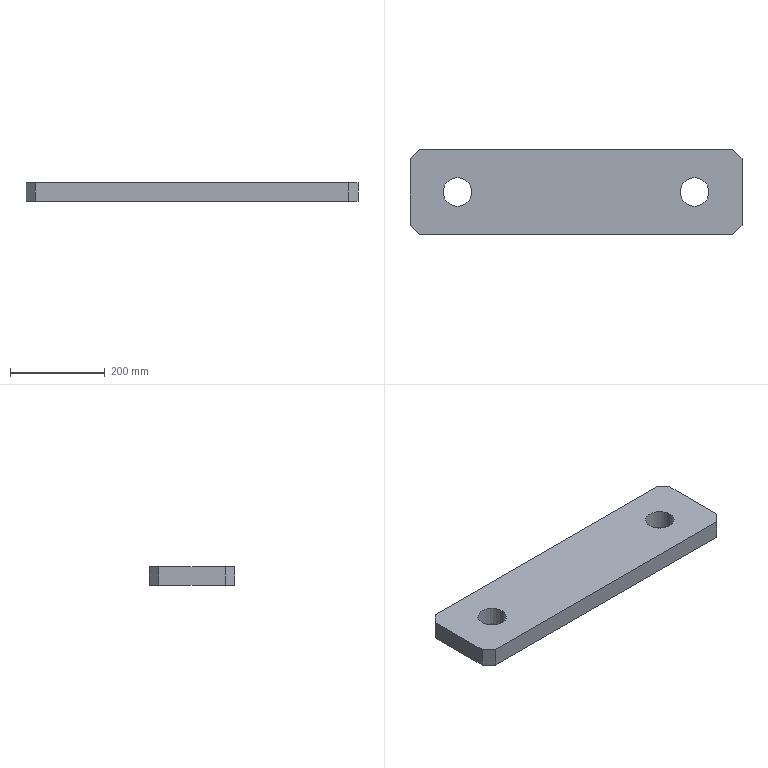Part | STEP file | 001-009-Riveting base plate | 1 solid | 14 faces | box 700 x 180 x 40 mm | volume 4781805 mm3 | plane 10 | cylinder 4 | commonest cylinder face diameters 60 x4
STEP:
#1=CARTESIAN_POINT('',(0.,0.,0.));
#2=DIRECTION('',(0.,0.,1.));
#3=DIRECTION('',(1.,0.,0.));
#4=AXIS2_PLACEMENT_3D('',#1,#2,#3);
#5=CARTESIAN_POINT('',(220.,0.,40.));
#6=VERTEX_POINT('',#5);
#7=CARTESIAN_POINT('',(220.,0.,0.));
#8=VERTEX_POINT('',#7);
#9=CARTESIAN_POINT('',(220.,0.,40.));
#10=DIRECTION('',(0.,0.,-1.));
#11=VECTOR('',#10,1.);
#12=LINE('',#9,#11);
#13=CARTESIAN_POINT('',(250.,0.,40.));
#14=DIRECTION('',(0.,0.,-1.));
#15=DIRECTION('',(-1.,0.,0.));
#16=AXIS2_PLACEMENT_3D('',#13,#14,#15);
#17=CYLINDRICAL_SURFACE('',#16,30.);
#18=CARTESIAN_POINT('',(6.283,0.));
#19=DIRECTION('',(0.,1.));
#20=VECTOR('',#19,1.);
#21=LINE('',#18,#20);
#22=(GEOMETRIC_REPRESENTATION_CONTEXT(2)PARAMETRIC_REPRESENTATION_CONTEXT()REPRESENTATION_CONTEXT('',''));
#23=DEFINITIONAL_REPRESENTATION('',(#21),#22);
#24=PCURVE('',#17,#23);
#25=CARTESIAN_POINT('',(250.,0.,40.));
#26=DIRECTION('',(0.,0.,-1.));
#27=DIRECTION('',(-1.,0.,0.));
#28=AXIS2_PLACEMENT_3D('',#25,#26,#27);
#29=CYLINDRICAL_SURFACE('',#28,30.);
#30=CARTESIAN_POINT('',(0.,0.));
#31=DIRECTION('',(0.,1.));
#32=VECTOR('',#31,1.);
#33=LINE('',#30,#32);
#34=(GEOMETRIC_REPRESENTATION_CONTEXT(2)PARAMETRIC_REPRESENTATION_CONTEXT()REPRESENTATION_CONTEXT('',''));
#35=DEFINITIONAL_REPRESENTATION('',(#33),#34);
#36=PCURVE('',#29,#35);
#37=SURFACE_CURVE('',#12,(#24,#36),.PCURVE_S1.);
#38=EDGE_CURVE('',#6,#8,#37,.T.);
#39=ORIENTED_EDGE('',*,*,#38,.T.);
#40=CARTESIAN_POINT('',(280.,0.,0.));
#41=VERTEX_POINT('',#40);
#42=CARTESIAN_POINT('',(250.,0.,0.));
#43=DIRECTION('',(0.,0.,-1.));
#44=DIRECTION('',(-1.,0.,0.));
#45=AXIS2_PLACEMENT_3D('',#42,#43,#44);
#46=CIRCLE('',#45,30.);
#47=CARTESIAN_POINT('',(0.,40.));
#48=DIRECTION('',(1.,0.));
#49=VECTOR('',#48,1.);
#50=LINE('',#47,#49);
#51=(GEOMETRIC_REPRESENTATION_CONTEXT(2)PARAMETRIC_REPRESENTATION_CONTEXT()REPRESENTATION_CONTEXT('',''));
#52=DEFINITIONAL_REPRESENTATION('',(#50),#51);
#53=PCURVE('',#17,#52);
#54=CARTESIAN_POINT('',(0.,0.,0.));
#55=DIRECTION('',(0.,0.,-1.));
#56=DIRECTION('',(-1.,0.,0.));
#57=AXIS2_PLACEMENT_3D('',#54,#55,#56);
#58=PLANE('',#57);
#59=CARTESIAN_POINT('',(-250.,0.));
#60=DIRECTION('',(1.,0.));
#61=AXIS2_PLACEMENT_2D('',#59,#60);
#62=CIRCLE('',#61,30.);
#63=(GEOMETRIC_REPRESENTATION_CONTEXT(2)PARAMETRIC_REPRESENTATION_CONTEXT()REPRESENTATION_CONTEXT('',''));
#64=DEFINITIONAL_REPRESENTATION('',(#62),#63);
#65=PCURVE('',#58,#64);
#66=SURFACE_CURVE('',#46,(#53,#65),.PCURVE_S1.);
#67=EDGE_CURVE('',#41,#8,#66,.T.);
#68=ORIENTED_EDGE('',*,*,#67,.F.);
#69=CARTESIAN_POINT('',(280.,0.,40.));
#70=VERTEX_POINT('',#69);
#71=CARTESIAN_POINT('',(280.,0.,40.));
#72=DIRECTION('',(0.,0.,-1.));
#73=VECTOR('',#72,1.);
#74=LINE('',#71,#73);
#75=CARTESIAN_POINT('',(3.142,0.));
#76=DIRECTION('',(0.,1.));
#77=VECTOR('',#76,1.);
#78=LINE('',#75,#77);
#79=(GEOMETRIC_REPRESENTATION_CONTEXT(2)PARAMETRIC_REPRESENTATION_CONTEXT()REPRESENTATION_CONTEXT('',''));
#80=DEFINITIONAL_REPRESENTATION('',(#78),#79);
#81=PCURVE('',#17,#80);
#82=CARTESIAN_POINT('',(3.142,0.));
#83=DIRECTION('',(0.,1.));
#84=VECTOR('',#83,1.);
#85=LINE('',#82,#84);
#86=(GEOMETRIC_REPRESENTATION_CONTEXT(2)PARAMETRIC_REPRESENTATION_CONTEXT()REPRESENTATION_CONTEXT('',''));
#87=DEFINITIONAL_REPRESENTATION('',(#85),#86);
#88=PCURVE('',#29,#87);
#89=SURFACE_CURVE('',#74,(#81,#88),.PCURVE_S1.);
#90=EDGE_CURVE('',#70,#41,#89,.T.);
#91=ORIENTED_EDGE('',*,*,#90,.F.);
#92=CARTESIAN_POINT('',(250.,0.,40.));
#93=DIRECTION('',(0.,0.,-1.));
#94=DIRECTION('',(-1.,0.,0.));
#95=AXIS2_PLACEMENT_3D('',#92,#93,#94);
#96=CIRCLE('',#95,30.);
#97=CARTESIAN_POINT('',(0.,0.));
#98=DIRECTION('',(1.,0.));
#99=VECTOR('',#98,1.);
#100=LINE('',#97,#99);
#101=(GEOMETRIC_REPRESENTATION_CONTEXT(2)PARAMETRIC_REPRESENTATION_CONTEXT()REPRESENTATION_CONTEXT('',''));
#102=DEFINITIONAL_REPRESENTATION('',(#100),#101);
#103=PCURVE('',#17,#102);
#104=CARTESIAN_POINT('',(0.,0.,40.));
#105=DIRECTION('',(0.,0.,-1.));
#106=DIRECTION('',(-1.,0.,0.));
#107=AXIS2_PLACEMENT_3D('',#104,#105,#106);
#108=PLANE('',#107);
#109=CARTESIAN_POINT('',(-250.,0.));
#110=DIRECTION('',(1.,0.));
#111=AXIS2_PLACEMENT_2D('',#109,#110);
#112=CIRCLE('',#111,30.);
#113=(GEOMETRIC_REPRESENTATION_CONTEXT(2)PARAMETRIC_REPRESENTATION_CONTEXT()REPRESENTATION_CONTEXT('',''));
#114=DEFINITIONAL_REPRESENTATION('',(#112),#113);
#115=PCURVE('',#108,#114);
#116=SURFACE_CURVE('',#96,(#103,#115),.PCURVE_S1.);
#117=EDGE_CURVE('',#70,#6,#116,.T.);
#118=ORIENTED_EDGE('',*,*,#117,.T.);
#119=EDGE_LOOP('',(#39,#68,#91,#118));
#120=FACE_BOUND('',#119,.F.);
#121=ADVANCED_FACE('',(#120),#17,.F.);
#122=CARTESIAN_POINT('',(-280.,0.,40.));
#123=VERTEX_POINT('',#122);
#124=CARTESIAN_POINT('',(-280.,0.,0.));
#125=VERTEX_POINT('',#124);
#126=CARTESIAN_POINT('',(-280.,0.,40.));
#127=DIRECTION('',(0.,0.,-1.));
#128=VECTOR('',#127,1.);
#129=LINE('',#126,#128);
#130=CARTESIAN_POINT('',(-250.,0.,40.));
#131=DIRECTION('',(0.,0.,-1.));
#132=DIRECTION('',(-1.,0.,0.));
#133=AXIS2_PLACEMENT_3D('',#130,#131,#132);
#134=CYLINDRICAL_SURFACE('',#133,30.);
#135=CARTESIAN_POINT('',(6.283,0.));
#136=DIRECTION('',(0.,1.));
#137=VECTOR('',#136,1.);
#138=LINE('',#135,#137);
#139=(GEOMETRIC_REPRESENTATION_CONTEXT(2)PARAMETRIC_REPRESENTATION_CONTEXT()REPRESENTATION_CONTEXT('',''));
#140=DEFINITIONAL_REPRESENTATION('',(#138),#139);
#141=PCURVE('',#134,#140);
#142=CARTESIAN_POINT('',(-250.,0.,40.));
#143=DIRECTION('',(0.,0.,-1.));
#144=DIRECTION('',(-1.,0.,0.));
#145=AXIS2_PLACEMENT_3D('',#142,#143,#144);
#146=CYLINDRICAL_SURFACE('',#145,30.);
#147=CARTESIAN_POINT('',(0.,0.));
#148=DIRECTION('',(0.,1.));
#149=VECTOR('',#148,1.);
#150=LINE('',#147,#149);
#151=(GEOMETRIC_REPRESENTATION_CONTEXT(2)PARAMETRIC_REPRESENTATION_CONTEXT()REPRESENTATION_CONTEXT('',''));
#152=DEFINITIONAL_REPRESENTATION('',(#150),#151);
#153=PCURVE('',#146,#152);
#154=SURFACE_CURVE('',#129,(#141,#153),.PCURVE_S1.);
#155=EDGE_CURVE('',#123,#125,#154,.T.);
#156=ORIENTED_EDGE('',*,*,#155,.T.);
#157=CARTESIAN_POINT('',(-220.,0.,0.));
#158=VERTEX_POINT('',#157);
#159=CARTESIAN_POINT('',(-250.,0.,0.));
#160=DIRECTION('',(0.,0.,-1.));
#161=DIRECTION('',(1.,0.,0.));
#162=AXIS2_PLACEMENT_3D('',#159,#160,#161);
#163=CIRCLE('',#162,30.);
#164=CARTESIAN_POINT('',(3.142,40.));
#165=DIRECTION('',(1.,0.));
#166=VECTOR('',#165,1.);
#167=LINE('',#164,#166);
#168=(GEOMETRIC_REPRESENTATION_CONTEXT(2)PARAMETRIC_REPRESENTATION_CONTEXT()REPRESENTATION_CONTEXT('',''));
#169=DEFINITIONAL_REPRESENTATION('',(#167),#168);
#170=PCURVE('',#134,#169);
#171=CARTESIAN_POINT('',(250.,0.));
#172=DIRECTION('',(-1.,0.));
#173=AXIS2_PLACEMENT_2D('',#171,#172);
#174=CIRCLE('',#173,30.);
#175=(GEOMETRIC_REPRESENTATION_CONTEXT(2)PARAMETRIC_REPRESENTATION_CONTEXT()REPRESENTATION_CONTEXT('',''));
#176=DEFINITIONAL_REPRESENTATION('',(#174),#175);
#177=PCURVE('',#58,#176);
#178=SURFACE_CURVE('',#163,(#170,#177),.PCURVE_S1.);
#179=EDGE_CURVE('',#158,#125,#178,.T.);
#180=ORIENTED_EDGE('',*,*,#179,.F.);
#181=CARTESIAN_POINT('',(-220.,0.,40.));
#182=VERTEX_POINT('',#181);
#183=CARTESIAN_POINT('',(-220.,0.,40.));
#184=DIRECTION('',(0.,0.,-1.));
#185=VECTOR('',#184,1.);
#186=LINE('',#183,#185);
#187=CARTESIAN_POINT('',(3.142,0.));
#188=DIRECTION('',(0.,1.));
#189=VECTOR('',#188,1.);
#190=LINE('',#187,#189);
#191=(GEOMETRIC_REPRESENTATION_CONTEXT(2)PARAMETRIC_REPRESENTATION_CONTEXT()REPRESENTATION_CONTEXT('',''));
#192=DEFINITIONAL_REPRESENTATION('',(#190),#191);
#193=PCURVE('',#134,#192);
#194=CARTESIAN_POINT('',(3.142,0.));
#195=DIRECTION('',(0.,1.));
#196=VECTOR('',#195,1.);
#197=LINE('',#194,#196);
#198=(GEOMETRIC_REPRESENTATION_CONTEXT(2)PARAMETRIC_REPRESENTATION_CONTEXT()REPRESENTATION_CONTEXT('',''));
#199=DEFINITIONAL_REPRESENTATION('',(#197),#198);
#200=PCURVE('',#146,#199);
#201=SURFACE_CURVE('',#186,(#193,#200),.PCURVE_S1.);
#202=EDGE_CURVE('',#182,#158,#201,.T.);
#203=ORIENTED_EDGE('',*,*,#202,.F.);
#204=CARTESIAN_POINT('',(-250.,0.,40.));
#205=DIRECTION('',(0.,0.,-1.));
#206=DIRECTION('',(1.,0.,0.));
#207=AXIS2_PLACEMENT_3D('',#204,#205,#206);
#208=CIRCLE('',#207,30.);
#209=CARTESIAN_POINT('',(3.142,0.));
#210=DIRECTION('',(1.,0.));
#211=VECTOR('',#210,1.);
#212=LINE('',#209,#211);
#213=(GEOMETRIC_REPRESENTATION_CONTEXT(2)PARAMETRIC_REPRESENTATION_CONTEXT()REPRESENTATION_CONTEXT('',''));
#214=DEFINITIONAL_REPRESENTATION('',(#212),#213);
#215=PCURVE('',#134,#214);
#216=CARTESIAN_POINT('',(250.,0.));
#217=DIRECTION('',(-1.,0.));
#218=AXIS2_PLACEMENT_2D('',#216,#217);
#219=CIRCLE('',#218,30.);
#220=(GEOMETRIC_REPRESENTATION_CONTEXT(2)PARAMETRIC_REPRESENTATION_CONTEXT()REPRESENTATION_CONTEXT('',''));
#221=DEFINITIONAL_REPRESENTATION('',(#219),#220);
#222=PCURVE('',#108,#221);
#223=SURFACE_CURVE('',#208,(#215,#222),.PCURVE_S1.);
#224=EDGE_CURVE('',#182,#123,#223,.T.);
#225=ORIENTED_EDGE('',*,*,#224,.T.);
#226=EDGE_LOOP('',(#156,#180,#203,#225));
#227=FACE_BOUND('',#226,.F.);
#228=ADVANCED_FACE('',(#227),#134,.F.);
#229=CARTESIAN_POINT('',(350.,-70.,0.));
#230=VERTEX_POINT('',#229);
#231=CARTESIAN_POINT('',(350.,70.,0.));
#232=VERTEX_POINT('',#231);
#233=CARTESIAN_POINT('',(350.,-90.,0.));
#234=DIRECTION('',(0.,1.,0.));
#235=VECTOR('',#234,1.);
#236=LINE('',#233,#235);
#237=CARTESIAN_POINT('',(350.,-90.,40.));
#238=DIRECTION('',(-1.,0.,0.));
#239=DIRECTION('',(0.,-1.,0.));
#240=AXIS2_PLACEMENT_3D('',#237,#238,#239);
#241=PLANE('',#240);
#242=CARTESIAN_POINT('',(0.,-40.));
#243=DIRECTION('',(-1.,0.));
#244=VECTOR('',#243,1.);
#245=LINE('',#242,#244);
#246=(GEOMETRIC_REPRESENTATION_CONTEXT(2)PARAMETRIC_REPRESENTATION_CONTEXT()REPRESENTATION_CONTEXT('',''));
#247=DEFINITIONAL_REPRESENTATION('',(#245),#246);
#248=PCURVE('',#241,#247);
#249=CARTESIAN_POINT('',(-350.,-90.));
#250=DIRECTION('',(0.,1.));
#251=VECTOR('',#250,1.);
#252=LINE('',#249,#251);
#253=(GEOMETRIC_REPRESENTATION_CONTEXT(2)PARAMETRIC_REPRESENTATION_CONTEXT()REPRESENTATION_CONTEXT('',''));
#254=DEFINITIONAL_REPRESENTATION('',(#252),#253);
#255=PCURVE('',#58,#254);
#256=SURFACE_CURVE('',#236,(#248,#255),.PCURVE_S1.);
#257=EDGE_CURVE('',#230,#232,#256,.T.);
#258=ORIENTED_EDGE('',*,*,#257,.T.);
#259=CARTESIAN_POINT('',(350.,70.,40.));
#260=VERTEX_POINT('',#259);
#261=CARTESIAN_POINT('',(350.,70.,40.));
#262=DIRECTION('',(0.,0.,1.));
#263=VECTOR('',#262,1.);
#264=LINE('',#261,#263);
#265=CARTESIAN_POINT('',(-160.,0.));
#266=DIRECTION('',(0.,1.));
#267=VECTOR('',#266,1.);
#268=LINE('',#265,#267);
#269=(GEOMETRIC_REPRESENTATION_CONTEXT(2)PARAMETRIC_REPRESENTATION_CONTEXT()REPRESENTATION_CONTEXT('',''));
#270=DEFINITIONAL_REPRESENTATION('',(#268),#269);
#271=PCURVE('',#241,#270);
#272=CARTESIAN_POINT('',(330.,90.,40.));
#273=DIRECTION('',(-0.7071,-0.7071,0.));
#274=DIRECTION('',(0.,0.,-1.));
#275=AXIS2_PLACEMENT_3D('',#272,#273,#274);
#276=PLANE('',#275);
#277=CARTESIAN_POINT('',(0.,28.284));
#278=DIRECTION('',(-1.,0.));
#279=VECTOR('',#278,1.);
#280=LINE('',#277,#279);
#281=(GEOMETRIC_REPRESENTATION_CONTEXT(2)PARAMETRIC_REPRESENTATION_CONTEXT()REPRESENTATION_CONTEXT('',''));
#282=DEFINITIONAL_REPRESENTATION('',(#280),#281);
#283=PCURVE('',#276,#282);
#284=SURFACE_CURVE('',#264,(#271,#283),.PCURVE_S1.);
#285=EDGE_CURVE('',#232,#260,#284,.T.);
#286=ORIENTED_EDGE('',*,*,#285,.T.);
#287=CARTESIAN_POINT('',(350.,-70.,40.));
#288=VERTEX_POINT('',#287);
#289=CARTESIAN_POINT('',(350.,-90.,40.));
#290=DIRECTION('',(0.,1.,0.));
#291=VECTOR('',#290,1.);
#292=LINE('',#289,#291);
#293=CARTESIAN_POINT('',(0.,0.));
#294=DIRECTION('',(-1.,0.));
#295=VECTOR('',#294,1.);
#296=LINE('',#293,#295);
#297=(GEOMETRIC_REPRESENTATION_CONTEXT(2)PARAMETRIC_REPRESENTATION_CONTEXT()REPRESENTATION_CONTEXT('',''));
#298=DEFINITIONAL_REPRESENTATION('',(#296),#297);
#299=PCURVE('',#241,#298);
#300=CARTESIAN_POINT('',(-350.,-90.));
#301=DIRECTION('',(0.,1.));
#302=VECTOR('',#301,1.);
#303=LINE('',#300,#302);
#304=(GEOMETRIC_REPRESENTATION_CONTEXT(2)PARAMETRIC_REPRESENTATION_CONTEXT()REPRESENTATION_CONTEXT('',''));
#305=DEFINITIONAL_REPRESENTATION('',(#303),#304);
#306=PCURVE('',#108,#305);
#307=SURFACE_CURVE('',#292,(#299,#306),.PCURVE_S1.);
#308=EDGE_CURVE('',#288,#260,#307,.T.);
#309=ORIENTED_EDGE('',*,*,#308,.F.);
#310=CARTESIAN_POINT('',(350.,-70.,40.));
#311=DIRECTION('',(0.,0.,-1.));
#312=VECTOR('',#311,1.);
#313=LINE('',#310,#312);
#314=CARTESIAN_POINT('',(-20.,0.));
#315=DIRECTION('',(0.,-1.));
#316=VECTOR('',#315,1.);
#317=LINE('',#314,#316);
#318=(GEOMETRIC_REPRESENTATION_CONTEXT(2)PARAMETRIC_REPRESENTATION_CONTEXT()REPRESENTATION_CONTEXT('',''));
#319=DEFINITIONAL_REPRESENTATION('',(#317),#318);
#320=PCURVE('',#241,#319);
#321=CARTESIAN_POINT('',(350.,-70.,40.));
#322=DIRECTION('',(-0.7071,0.7071,0.));
#323=DIRECTION('',(0.,0.,-1.));
#324=AXIS2_PLACEMENT_3D('',#321,#322,#323);
#325=PLANE('',#324);
#326=CARTESIAN_POINT('',(0.,0.));
#327=DIRECTION('',(1.,0.));
#328=VECTOR('',#327,1.);
#329=LINE('',#326,#328);
#330=(GEOMETRIC_REPRESENTATION_CONTEXT(2)PARAMETRIC_REPRESENTATION_CONTEXT()REPRESENTATION_CONTEXT('',''));
#331=DEFINITIONAL_REPRESENTATION('',(#329),#330);
#332=PCURVE('',#325,#331);
#333=SURFACE_CURVE('',#313,(#320,#332),.PCURVE_S1.);
#334=EDGE_CURVE('',#288,#230,#333,.T.);
#335=ORIENTED_EDGE('',*,*,#334,.T.);
#336=EDGE_LOOP('',(#258,#286,#309,#335));
#337=FACE_BOUND('',#336,.T.);
#338=ADVANCED_FACE('',(#337),#241,.F.);
#339=CARTESIAN_POINT('',(330.,90.,0.));
#340=VERTEX_POINT('',#339);
#341=CARTESIAN_POINT('',(-330.,90.,0.));
#342=VERTEX_POINT('',#341);
#343=CARTESIAN_POINT('',(-350.,90.,0.));
#344=DIRECTION('',(-1.,0.,0.));
#345=VECTOR('',#344,1.);
#346=LINE('',#343,#345);
#347=CARTESIAN_POINT('',(-350.,90.,40.));
#348=DIRECTION('',(0.,-1.,0.));
#349=DIRECTION('',(0.,0.,-1.));
#350=AXIS2_PLACEMENT_3D('',#347,#348,#349);
#351=PLANE('',#350);
#352=CARTESIAN_POINT('',(40.,0.));
#353=DIRECTION('',(0.,-1.));
#354=VECTOR('',#353,1.);
#355=LINE('',#352,#354);
#356=(GEOMETRIC_REPRESENTATION_CONTEXT(2)PARAMETRIC_REPRESENTATION_CONTEXT()REPRESENTATION_CONTEXT('',''));
#357=DEFINITIONAL_REPRESENTATION('',(#355),#356);
#358=PCURVE('',#351,#357);
#359=CARTESIAN_POINT('',(350.,90.));
#360=DIRECTION('',(1.,0.));
#361=VECTOR('',#360,1.);
#362=LINE('',#359,#361);
#363=(GEOMETRIC_REPRESENTATION_CONTEXT(2)PARAMETRIC_REPRESENTATION_CONTEXT()REPRESENTATION_CONTEXT('',''));
#364=DEFINITIONAL_REPRESENTATION('',(#362),#363);
#365=PCURVE('',#58,#364);
#366=SURFACE_CURVE('',#346,(#358,#365),.PCURVE_S1.);
#367=EDGE_CURVE('',#340,#342,#366,.T.);
#368=ORIENTED_EDGE('',*,*,#367,.T.);
#369=CARTESIAN_POINT('',(-330.,90.,40.));
#370=VERTEX_POINT('',#369);
#371=CARTESIAN_POINT('',(-330.,90.,40.));
#372=DIRECTION('',(0.,0.,1.));
#373=VECTOR('',#372,1.);
#374=LINE('',#371,#373);
#375=CARTESIAN_POINT('',(0.,20.));
#376=DIRECTION('',(-1.,0.));
#377=VECTOR('',#376,1.);
#378=LINE('',#375,#377);
#379=(GEOMETRIC_REPRESENTATION_CONTEXT(2)PARAMETRIC_REPRESENTATION_CONTEXT()REPRESENTATION_CONTEXT('',''));
#380=DEFINITIONAL_REPRESENTATION('',(#378),#379);
#381=PCURVE('',#351,#380);
#382=CARTESIAN_POINT('',(-350.,70.,40.));
#383=DIRECTION('',(0.7071,-0.7071,0.));
#384=DIRECTION('',(0.,0.,-1.));
#385=AXIS2_PLACEMENT_3D('',#382,#383,#384);
#386=PLANE('',#385);
#387=CARTESIAN_POINT('',(0.,28.284));
#388=DIRECTION('',(-1.,0.));
#389=VECTOR('',#388,1.);
#390=LINE('',#387,#389);
#391=(GEOMETRIC_REPRESENTATION_CONTEXT(2)PARAMETRIC_REPRESENTATION_CONTEXT()REPRESENTATION_CONTEXT('',''));
#392=DEFINITIONAL_REPRESENTATION('',(#390),#391);
#393=PCURVE('',#386,#392);
#394=SURFACE_CURVE('',#374,(#381,#393),.PCURVE_S1.);
#395=EDGE_CURVE('',#342,#370,#394,.T.);
#396=ORIENTED_EDGE('',*,*,#395,.T.);
#397=CARTESIAN_POINT('',(330.,90.,40.));
#398=VERTEX_POINT('',#397);
#399=CARTESIAN_POINT('',(-350.,90.,40.));
#400=DIRECTION('',(-1.,0.,0.));
#401=VECTOR('',#400,1.);
#402=LINE('',#399,#401);
#403=CARTESIAN_POINT('',(0.,0.));
#404=DIRECTION('',(0.,-1.));
#405=VECTOR('',#404,1.);
#406=LINE('',#403,#405);
#407=(GEOMETRIC_REPRESENTATION_CONTEXT(2)PARAMETRIC_REPRESENTATION_CONTEXT()REPRESENTATION_CONTEXT('',''));
#408=DEFINITIONAL_REPRESENTATION('',(#406),#407);
#409=PCURVE('',#351,#408);
#410=CARTESIAN_POINT('',(350.,90.));
#411=DIRECTION('',(1.,0.));
#412=VECTOR('',#411,1.);
#413=LINE('',#410,#412);
#414=(GEOMETRIC_REPRESENTATION_CONTEXT(2)PARAMETRIC_REPRESENTATION_CONTEXT()REPRESENTATION_CONTEXT('',''));
#415=DEFINITIONAL_REPRESENTATION('',(#413),#414);
#416=PCURVE('',#108,#415);
#417=SURFACE_CURVE('',#402,(#409,#416),.PCURVE_S1.);
#418=EDGE_CURVE('',#398,#370,#417,.T.);
#419=ORIENTED_EDGE('',*,*,#418,.F.);
#420=CARTESIAN_POINT('',(330.,90.,40.));
#421=DIRECTION('',(0.,0.,-1.));
#422=VECTOR('',#421,1.);
#423=LINE('',#420,#422);
#424=CARTESIAN_POINT('',(0.,680.));
#425=DIRECTION('',(1.,0.));
#426=VECTOR('',#425,1.);
#427=LINE('',#424,#426);
#428=(GEOMETRIC_REPRESENTATION_CONTEXT(2)PARAMETRIC_REPRESENTATION_CONTEXT()REPRESENTATION_CONTEXT('',''));
#429=DEFINITIONAL_REPRESENTATION('',(#427),#428);
#430=PCURVE('',#351,#429);
#431=CARTESIAN_POINT('',(0.,0.));
#432=DIRECTION('',(1.,0.));
#433=VECTOR('',#432,1.);
#434=LINE('',#431,#433);
#435=(GEOMETRIC_REPRESENTATION_CONTEXT(2)PARAMETRIC_REPRESENTATION_CONTEXT()REPRESENTATION_CONTEXT('',''));
#436=DEFINITIONAL_REPRESENTATION('',(#434),#435);
#437=PCURVE('',#276,#436);
#438=SURFACE_CURVE('',#423,(#430,#437),.PCURVE_S1.);
#439=EDGE_CURVE('',#398,#340,#438,.T.);
#440=ORIENTED_EDGE('',*,*,#439,.T.);
#441=EDGE_LOOP('',(#368,#396,#419,#440));
#442=FACE_BOUND('',#441,.T.);
#443=ADVANCED_FACE('',(#442),#351,.F.);
#444=CARTESIAN_POINT('',(-350.,70.,0.));
#445=VERTEX_POINT('',#444);
#446=CARTESIAN_POINT('',(-350.,-70.,0.));
#447=VERTEX_POINT('',#446);
#448=CARTESIAN_POINT('',(-350.,-90.,0.));
#449=DIRECTION('',(0.,-1.,0.));
#450=VECTOR('',#449,1.);
#451=LINE('',#448,#450);
#452=CARTESIAN_POINT('',(-350.,-90.,40.));
#453=DIRECTION('',(1.,0.,0.));
#454=DIRECTION('',(0.,0.,-1.));
#455=AXIS2_PLACEMENT_3D('',#452,#453,#454);
#456=PLANE('',#455);
#457=CARTESIAN_POINT('',(40.,0.));
#458=DIRECTION('',(0.,-1.));
#459=VECTOR('',#458,1.);
#460=LINE('',#457,#459);
#461=(GEOMETRIC_REPRESENTATION_CONTEXT(2)PARAMETRIC_REPRESENTATION_CONTEXT()REPRESENTATION_CONTEXT('',''));
#462=DEFINITIONAL_REPRESENTATION('',(#460),#461);
#463=PCURVE('',#456,#462);
#464=CARTESIAN_POINT('',(350.,-90.));
#465=DIRECTION('',(0.,-1.));
#466=VECTOR('',#465,1.);
#467=LINE('',#464,#466);
#468=(GEOMETRIC_REPRESENTATION_CONTEXT(2)PARAMETRIC_REPRESENTATION_CONTEXT()REPRESENTATION_CONTEXT('',''));
#469=DEFINITIONAL_REPRESENTATION('',(#467),#468);
#470=PCURVE('',#58,#469);
#471=SURFACE_CURVE('',#451,(#463,#470),.PCURVE_S1.);
#472=EDGE_CURVE('',#445,#447,#471,.T.);
#473=ORIENTED_EDGE('',*,*,#472,.T.);
#474=CARTESIAN_POINT('',(-350.,-70.,40.));
#475=VERTEX_POINT('',#474);
#476=CARTESIAN_POINT('',(-350.,-70.,40.));
#477=DIRECTION('',(0.,0.,1.));
#478=VECTOR('',#477,1.);
#479=LINE('',#476,#478);
#480=CARTESIAN_POINT('',(0.,20.));
#481=DIRECTION('',(-1.,0.));
#482=VECTOR('',#481,1.);
#483=LINE('',#480,#482);
#484=(GEOMETRIC_REPRESENTATION_CONTEXT(2)PARAMETRIC_REPRESENTATION_CONTEXT()REPRESENTATION_CONTEXT('',''));
#485=DEFINITIONAL_REPRESENTATION('',(#483),#484);
#486=PCURVE('',#456,#485);
#487=CARTESIAN_POINT('',(-330.,-90.,40.));
#488=DIRECTION('',(0.7071,0.7071,0.));
#489=DIRECTION('',(0.,0.,-1.));
#490=AXIS2_PLACEMENT_3D('',#487,#488,#489);
#491=PLANE('',#490);
#492=CARTESIAN_POINT('',(0.,28.284));
#493=DIRECTION('',(-1.,0.));
#494=VECTOR('',#493,1.);
#495=LINE('',#492,#494);
#496=(GEOMETRIC_REPRESENTATION_CONTEXT(2)PARAMETRIC_REPRESENTATION_CONTEXT()REPRESENTATION_CONTEXT('',''));
#497=DEFINITIONAL_REPRESENTATION('',(#495),#496);
#498=PCURVE('',#491,#497);
#499=SURFACE_CURVE('',#479,(#486,#498),.PCURVE_S1.);
#500=EDGE_CURVE('',#447,#475,#499,.T.);
#501=ORIENTED_EDGE('',*,*,#500,.T.);
#502=CARTESIAN_POINT('',(-350.,70.,40.));
#503=VERTEX_POINT('',#502);
#504=CARTESIAN_POINT('',(-350.,-90.,40.));
#505=DIRECTION('',(0.,-1.,0.));
#506=VECTOR('',#505,1.);
#507=LINE('',#504,#506);
#508=CARTESIAN_POINT('',(0.,0.));
#509=DIRECTION('',(0.,-1.));
#510=VECTOR('',#509,1.);
#511=LINE('',#508,#510);
#512=(GEOMETRIC_REPRESENTATION_CONTEXT(2)PARAMETRIC_REPRESENTATION_CONTEXT()REPRESENTATION_CONTEXT('',''));
#513=DEFINITIONAL_REPRESENTATION('',(#511),#512);
#514=PCURVE('',#456,#513);
#515=CARTESIAN_POINT('',(350.,-90.));
#516=DIRECTION('',(0.,-1.));
#517=VECTOR('',#516,1.);
#518=LINE('',#515,#517);
#519=(GEOMETRIC_REPRESENTATION_CONTEXT(2)PARAMETRIC_REPRESENTATION_CONTEXT()REPRESENTATION_CONTEXT('',''));
#520=DEFINITIONAL_REPRESENTATION('',(#518),#519);
#521=PCURVE('',#108,#520);
#522=SURFACE_CURVE('',#507,(#514,#521),.PCURVE_S1.);
#523=EDGE_CURVE('',#503,#475,#522,.T.);
#524=ORIENTED_EDGE('',*,*,#523,.F.);
#525=CARTESIAN_POINT('',(-350.,70.,40.));
#526=DIRECTION('',(0.,0.,-1.));
#527=VECTOR('',#526,1.);
#528=LINE('',#525,#527);
#529=CARTESIAN_POINT('',(0.,160.));
#530=DIRECTION('',(1.,0.));
#531=VECTOR('',#530,1.);
#532=LINE('',#529,#531);
#533=(GEOMETRIC_REPRESENTATION_CONTEXT(2)PARAMETRIC_REPRESENTATION_CONTEXT()REPRESENTATION_CONTEXT('',''));
#534=DEFINITIONAL_REPRESENTATION('',(#532),#533);
#535=PCURVE('',#456,#534);
#536=CARTESIAN_POINT('',(0.,0.));
#537=DIRECTION('',(1.,0.));
#538=VECTOR('',#537,1.);
#539=LINE('',#536,#538);
#540=(GEOMETRIC_REPRESENTATION_CONTEXT(2)PARAMETRIC_REPRESENTATION_CONTEXT()REPRESENTATION_CONTEXT('',''));
#541=DEFINITIONAL_REPRESENTATION('',(#539),#540);
#542=PCURVE('',#386,#541);
#543=SURFACE_CURVE('',#528,(#535,#542),.PCURVE_S1.);
#544=EDGE_CURVE('',#503,#445,#543,.T.);
#545=ORIENTED_EDGE('',*,*,#544,.T.);
#546=EDGE_LOOP('',(#473,#501,#524,#545));
#547=FACE_BOUND('',#546,.T.);
#548=ADVANCED_FACE('',(#547),#456,.F.);
#549=CARTESIAN_POINT('',(-330.,-90.,40.));
#550=VERTEX_POINT('',#549);
#551=CARTESIAN_POINT('',(330.,-90.,40.));
#552=VERTEX_POINT('',#551);
#553=CARTESIAN_POINT('',(-350.,-90.,40.));
#554=DIRECTION('',(1.,0.,0.));
#555=VECTOR('',#554,1.);
#556=LINE('',#553,#555);
#557=CARTESIAN_POINT('',(-350.,-90.,40.));
#558=DIRECTION('',(0.,1.,0.));
#559=DIRECTION('',(-1.,0.,0.));
#560=AXIS2_PLACEMENT_3D('',#557,#558,#559);
#561=PLANE('',#560);
#562=CARTESIAN_POINT('',(0.,0.));
#563=DIRECTION('',(-1.,0.));
#564=VECTOR('',#563,1.);
#565=LINE('',#562,#564);
#566=(GEOMETRIC_REPRESENTATION_CONTEXT(2)PARAMETRIC_REPRESENTATION_CONTEXT()REPRESENTATION_CONTEXT('',''));
#567=DEFINITIONAL_REPRESENTATION('',(#565),#566);
#568=PCURVE('',#561,#567);
#569=CARTESIAN_POINT('',(350.,-90.));
#570=DIRECTION('',(-1.,0.));
#571=VECTOR('',#570,1.);
#572=LINE('',#569,#571);
#573=(GEOMETRIC_REPRESENTATION_CONTEXT(2)PARAMETRIC_REPRESENTATION_CONTEXT()REPRESENTATION_CONTEXT('',''));
#574=DEFINITIONAL_REPRESENTATION('',(#572),#573);
#575=PCURVE('',#108,#574);
#576=SURFACE_CURVE('',#556,(#568,#575),.PCURVE_S1.);
#577=EDGE_CURVE('',#550,#552,#576,.T.);
#578=ORIENTED_EDGE('',*,*,#577,.F.);
#579=CARTESIAN_POINT('',(-330.,-90.,0.));
#580=VERTEX_POINT('',#579);
#581=CARTESIAN_POINT('',(-330.,-90.,40.));
#582=DIRECTION('',(0.,0.,-1.));
#583=VECTOR('',#582,1.);
#584=LINE('',#581,#583);
#585=CARTESIAN_POINT('',(-20.,0.));
#586=DIRECTION('',(0.,-1.));
#587=VECTOR('',#586,1.);
#588=LINE('',#585,#587);
#589=(GEOMETRIC_REPRESENTATION_CONTEXT(2)PARAMETRIC_REPRESENTATION_CONTEXT()REPRESENTATION_CONTEXT('',''));
#590=DEFINITIONAL_REPRESENTATION('',(#588),#589);
#591=PCURVE('',#561,#590);
#592=CARTESIAN_POINT('',(0.,0.));
#593=DIRECTION('',(1.,0.));
#594=VECTOR('',#593,1.);
#595=LINE('',#592,#594);
#596=(GEOMETRIC_REPRESENTATION_CONTEXT(2)PARAMETRIC_REPRESENTATION_CONTEXT()REPRESENTATION_CONTEXT('',''));
#597=DEFINITIONAL_REPRESENTATION('',(#595),#596);
#598=PCURVE('',#491,#597);
#599=SURFACE_CURVE('',#584,(#591,#598),.PCURVE_S1.);
#600=EDGE_CURVE('',#550,#580,#599,.T.);
#601=ORIENTED_EDGE('',*,*,#600,.T.);
#602=CARTESIAN_POINT('',(330.,-90.,0.));
#603=VERTEX_POINT('',#602);
#604=CARTESIAN_POINT('',(-350.,-90.,0.));
#605=DIRECTION('',(1.,0.,0.));
#606=VECTOR('',#605,1.);
#607=LINE('',#604,#606);
#608=CARTESIAN_POINT('',(0.,-40.));
#609=DIRECTION('',(-1.,0.));
#610=VECTOR('',#609,1.);
#611=LINE('',#608,#610);
#612=(GEOMETRIC_REPRESENTATION_CONTEXT(2)PARAMETRIC_REPRESENTATION_CONTEXT()REPRESENTATION_CONTEXT('',''));
#613=DEFINITIONAL_REPRESENTATION('',(#611),#612);
#614=PCURVE('',#561,#613);
#615=CARTESIAN_POINT('',(350.,-90.));
#616=DIRECTION('',(-1.,0.));
#617=VECTOR('',#616,1.);
#618=LINE('',#615,#617);
#619=(GEOMETRIC_REPRESENTATION_CONTEXT(2)PARAMETRIC_REPRESENTATION_CONTEXT()REPRESENTATION_CONTEXT('',''));
#620=DEFINITIONAL_REPRESENTATION('',(#618),#619);
#621=PCURVE('',#58,#620);
#622=SURFACE_CURVE('',#607,(#614,#621),.PCURVE_S1.);
#623=EDGE_CURVE('',#580,#603,#622,.T.);
#624=ORIENTED_EDGE('',*,*,#623,.T.);
#625=CARTESIAN_POINT('',(330.,-90.,40.));
#626=DIRECTION('',(0.,0.,1.));
#627=VECTOR('',#626,1.);
#628=LINE('',#625,#627);
#629=CARTESIAN_POINT('',(-680.,0.));
#630=DIRECTION('',(0.,1.));
#631=VECTOR('',#630,1.);
#632=LINE('',#629,#631);
#633=(GEOMETRIC_REPRESENTATION_CONTEXT(2)PARAMETRIC_REPRESENTATION_CONTEXT()REPRESENTATION_CONTEXT('',''));
#634=DEFINITIONAL_REPRESENTATION('',(#632),#633);
#635=PCURVE('',#561,#634);
#636=CARTESIAN_POINT('',(0.,28.284));
#637=DIRECTION('',(-1.,0.));
#638=VECTOR('',#637,1.);
#639=LINE('',#636,#638);
#640=(GEOMETRIC_REPRESENTATION_CONTEXT(2)PARAMETRIC_REPRESENTATION_CONTEXT()REPRESENTATION_CONTEXT('',''));
#641=DEFINITIONAL_REPRESENTATION('',(#639),#640);
#642=PCURVE('',#325,#641);
#643=SURFACE_CURVE('',#628,(#635,#642),.PCURVE_S1.);
#644=EDGE_CURVE('',#603,#552,#643,.T.);
#645=ORIENTED_EDGE('',*,*,#644,.T.);
#646=EDGE_LOOP('',(#578,#601,#624,#645));
#647=FACE_BOUND('',#646,.T.);
#648=ADVANCED_FACE('',(#647),#561,.F.);
#649=CARTESIAN_POINT('',(250.,0.,40.));
#650=DIRECTION('',(0.,0.,-1.));
#651=DIRECTION('',(-1.,0.,0.));
#652=AXIS2_PLACEMENT_3D('',#649,#650,#651);
#653=CIRCLE('',#652,30.);
#654=CARTESIAN_POINT('',(-250.,0.));
#655=DIRECTION('',(1.,0.));
#656=AXIS2_PLACEMENT_2D('',#654,#655);
#657=CIRCLE('',#656,30.);
#658=(GEOMETRIC_REPRESENTATION_CONTEXT(2)PARAMETRIC_REPRESENTATION_CONTEXT()REPRESENTATION_CONTEXT('',''));
#659=DEFINITIONAL_REPRESENTATION('',(#657),#658);
#660=PCURVE('',#108,#659);
#661=CARTESIAN_POINT('',(0.,0.));
#662=DIRECTION('',(1.,0.));
#663=VECTOR('',#662,1.);
#664=LINE('',#661,#663);
#665=(GEOMETRIC_REPRESENTATION_CONTEXT(2)PARAMETRIC_REPRESENTATION_CONTEXT()REPRESENTATION_CONTEXT('',''));
#666=DEFINITIONAL_REPRESENTATION('',(#664),#665);
#667=PCURVE('',#29,#666);
#668=SURFACE_CURVE('',#653,(#660,#667),.PCURVE_S1.);
#669=EDGE_CURVE('',#6,#70,#668,.T.);
#670=ORIENTED_EDGE('',*,*,#669,.T.);
#671=ORIENTED_EDGE('',*,*,#117,.T.);
#672=EDGE_LOOP('',(#670,#671));
#673=FACE_BOUND('',#672,.T.);
#674=CARTESIAN_POINT('',(-250.,0.,40.));
#675=DIRECTION('',(0.,0.,-1.));
#676=DIRECTION('',(1.,0.,0.));
#677=AXIS2_PLACEMENT_3D('',#674,#675,#676);
#678=CIRCLE('',#677,30.);
#679=CARTESIAN_POINT('',(250.,0.));
#680=DIRECTION('',(-1.,0.));
#681=AXIS2_PLACEMENT_2D('',#679,#680);
#682=CIRCLE('',#681,30.);
#683=(GEOMETRIC_REPRESENTATION_CONTEXT(2)PARAMETRIC_REPRESENTATION_CONTEXT()REPRESENTATION_CONTEXT('',''));
#684=DEFINITIONAL_REPRESENTATION('',(#682),#683);
#685=PCURVE('',#108,#684);
#686=CARTESIAN_POINT('',(-3.142,0.));
#687=DIRECTION('',(1.,0.));
#688=VECTOR('',#687,1.);
#689=LINE('',#686,#688);
#690=(GEOMETRIC_REPRESENTATION_CONTEXT(2)PARAMETRIC_REPRESENTATION_CONTEXT()REPRESENTATION_CONTEXT('',''));
#691=DEFINITIONAL_REPRESENTATION('',(#689),#690);
#692=PCURVE('',#146,#691);
#693=SURFACE_CURVE('',#678,(#685,#692),.PCURVE_S1.);
#694=EDGE_CURVE('',#123,#182,#693,.T.);
#695=ORIENTED_EDGE('',*,*,#694,.T.);
#696=ORIENTED_EDGE('',*,*,#224,.T.);
#697=EDGE_LOOP('',(#695,#696));
#698=FACE_BOUND('',#697,.T.);
#699=ORIENTED_EDGE('',*,*,#523,.T.);
#700=CARTESIAN_POINT('',(-330.,-90.,40.));
#701=DIRECTION('',(0.7071,-0.7071,0.));
#702=VECTOR('',#701,1.);
#703=LINE('',#700,#702);
#704=CARTESIAN_POINT('',(330.,-90.));
#705=DIRECTION('',(-0.7071,-0.7071));
#706=VECTOR('',#705,1.);
#707=LINE('',#704,#706);
#708=(GEOMETRIC_REPRESENTATION_CONTEXT(2)PARAMETRIC_REPRESENTATION_CONTEXT()REPRESENTATION_CONTEXT('',''));
#709=DEFINITIONAL_REPRESENTATION('',(#707),#708);
#710=PCURVE('',#108,#709);
#711=CARTESIAN_POINT('',(0.,0.));
#712=DIRECTION('',(0.,-1.));
#713=VECTOR('',#712,1.);
#714=LINE('',#711,#713);
#715=(GEOMETRIC_REPRESENTATION_CONTEXT(2)PARAMETRIC_REPRESENTATION_CONTEXT()REPRESENTATION_CONTEXT('',''));
#716=DEFINITIONAL_REPRESENTATION('',(#714),#715);
#717=PCURVE('',#491,#716);
#718=SURFACE_CURVE('',#703,(#710,#717),.PCURVE_S1.);
#719=EDGE_CURVE('',#475,#550,#718,.T.);
#720=ORIENTED_EDGE('',*,*,#719,.T.);
#721=ORIENTED_EDGE('',*,*,#577,.T.);
#722=CARTESIAN_POINT('',(350.,-70.,40.));
#723=DIRECTION('',(0.7071,0.7071,0.));
#724=VECTOR('',#723,1.);
#725=LINE('',#722,#724);
#726=CARTESIAN_POINT('',(-350.,-70.));
#727=DIRECTION('',(-0.7071,0.7071));
#728=VECTOR('',#727,1.);
#729=LINE('',#726,#728);
#730=(GEOMETRIC_REPRESENTATION_CONTEXT(2)PARAMETRIC_REPRESENTATION_CONTEXT()REPRESENTATION_CONTEXT('',''));
#731=DEFINITIONAL_REPRESENTATION('',(#729),#730);
#732=PCURVE('',#108,#731);
#733=CARTESIAN_POINT('',(0.,0.));
#734=DIRECTION('',(0.,-1.));
#735=VECTOR('',#734,1.);
#736=LINE('',#733,#735);
#737=(GEOMETRIC_REPRESENTATION_CONTEXT(2)PARAMETRIC_REPRESENTATION_CONTEXT()REPRESENTATION_CONTEXT('',''));
#738=DEFINITIONAL_REPRESENTATION('',(#736),#737);
#739=PCURVE('',#325,#738);
#740=SURFACE_CURVE('',#725,(#732,#739),.PCURVE_S1.);
#741=EDGE_CURVE('',#552,#288,#740,.T.);
#742=ORIENTED_EDGE('',*,*,#741,.T.);
#743=ORIENTED_EDGE('',*,*,#308,.T.);
#744=CARTESIAN_POINT('',(330.,90.,40.));
#745=DIRECTION('',(-0.7071,0.7071,0.));
#746=VECTOR('',#745,1.);
#747=LINE('',#744,#746);
#748=CARTESIAN_POINT('',(-330.,90.));
#749=DIRECTION('',(0.7071,0.7071));
#750=VECTOR('',#749,1.);
#751=LINE('',#748,#750);
#752=(GEOMETRIC_REPRESENTATION_CONTEXT(2)PARAMETRIC_REPRESENTATION_CONTEXT()REPRESENTATION_CONTEXT('',''));
#753=DEFINITIONAL_REPRESENTATION('',(#751),#752);
#754=PCURVE('',#108,#753);
#755=CARTESIAN_POINT('',(0.,0.));
#756=DIRECTION('',(0.,-1.));
#757=VECTOR('',#756,1.);
#758=LINE('',#755,#757);
#759=(GEOMETRIC_REPRESENTATION_CONTEXT(2)PARAMETRIC_REPRESENTATION_CONTEXT()REPRESENTATION_CONTEXT('',''));
#760=DEFINITIONAL_REPRESENTATION('',(#758),#759);
#761=PCURVE('',#276,#760);
#762=SURFACE_CURVE('',#747,(#754,#761),.PCURVE_S1.);
#763=EDGE_CURVE('',#260,#398,#762,.T.);
#764=ORIENTED_EDGE('',*,*,#763,.T.);
#765=ORIENTED_EDGE('',*,*,#418,.T.);
#766=CARTESIAN_POINT('',(-350.,70.,40.));
#767=DIRECTION('',(-0.7071,-0.7071,0.));
#768=VECTOR('',#767,1.);
#769=LINE('',#766,#768);
#770=CARTESIAN_POINT('',(350.,70.));
#771=DIRECTION('',(0.7071,-0.7071));
#772=VECTOR('',#771,1.);
#773=LINE('',#770,#772);
#774=(GEOMETRIC_REPRESENTATION_CONTEXT(2)PARAMETRIC_REPRESENTATION_CONTEXT()REPRESENTATION_CONTEXT('',''));
#775=DEFINITIONAL_REPRESENTATION('',(#773),#774);
#776=PCURVE('',#108,#775);
#777=CARTESIAN_POINT('',(0.,0.));
#778=DIRECTION('',(0.,-1.));
#779=VECTOR('',#778,1.);
#780=LINE('',#777,#779);
#781=(GEOMETRIC_REPRESENTATION_CONTEXT(2)PARAMETRIC_REPRESENTATION_CONTEXT()REPRESENTATION_CONTEXT('',''));
#782=DEFINITIONAL_REPRESENTATION('',(#780),#781);
#783=PCURVE('',#386,#782);
#784=SURFACE_CURVE('',#769,(#776,#783),.PCURVE_S1.);
#785=EDGE_CURVE('',#370,#503,#784,.T.);
#786=ORIENTED_EDGE('',*,*,#785,.T.);
#787=EDGE_LOOP('',(#699,#720,#721,#742,#743,#764,#765,#786));
#788=FACE_BOUND('',#787,.T.);
#789=ADVANCED_FACE('',(#673,#698,#788),#108,.F.);
#790=CARTESIAN_POINT('',(250.,0.,0.));
#791=DIRECTION('',(0.,0.,-1.));
#792=DIRECTION('',(-1.,0.,0.));
#793=AXIS2_PLACEMENT_3D('',#790,#791,#792);
#794=CIRCLE('',#793,30.);
#795=CARTESIAN_POINT('',(-250.,0.));
#796=DIRECTION('',(1.,0.));
#797=AXIS2_PLACEMENT_2D('',#795,#796);
#798=CIRCLE('',#797,30.);
#799=(GEOMETRIC_REPRESENTATION_CONTEXT(2)PARAMETRIC_REPRESENTATION_CONTEXT()REPRESENTATION_CONTEXT('',''));
#800=DEFINITIONAL_REPRESENTATION('',(#798),#799);
#801=PCURVE('',#58,#800);
#802=CARTESIAN_POINT('',(0.,40.));
#803=DIRECTION('',(1.,0.));
#804=VECTOR('',#803,1.);
#805=LINE('',#802,#804);
#806=(GEOMETRIC_REPRESENTATION_CONTEXT(2)PARAMETRIC_REPRESENTATION_CONTEXT()REPRESENTATION_CONTEXT('',''));
#807=DEFINITIONAL_REPRESENTATION('',(#805),#806);
#808=PCURVE('',#29,#807);
#809=SURFACE_CURVE('',#794,(#801,#808),.PCURVE_S1.);
#810=EDGE_CURVE('',#8,#41,#809,.T.);
#811=ORIENTED_EDGE('',*,*,#810,.F.);
#812=ORIENTED_EDGE('',*,*,#67,.F.);
#813=EDGE_LOOP('',(#811,#812));
#814=FACE_BOUND('',#813,.T.);
#815=CARTESIAN_POINT('',(-250.,0.,0.));
#816=DIRECTION('',(0.,0.,-1.));
#817=DIRECTION('',(1.,0.,0.));
#818=AXIS2_PLACEMENT_3D('',#815,#816,#817);
#819=CIRCLE('',#818,30.);
#820=CARTESIAN_POINT('',(250.,0.));
#821=DIRECTION('',(-1.,0.));
#822=AXIS2_PLACEMENT_2D('',#820,#821);
#823=CIRCLE('',#822,30.);
#824=(GEOMETRIC_REPRESENTATION_CONTEXT(2)PARAMETRIC_REPRESENTATION_CONTEXT()REPRESENTATION_CONTEXT('',''));
#825=DEFINITIONAL_REPRESENTATION('',(#823),#824);
#826=PCURVE('',#58,#825);
#827=CARTESIAN_POINT('',(-3.142,40.));
#828=DIRECTION('',(1.,0.));
#829=VECTOR('',#828,1.);
#830=LINE('',#827,#829);
#831=(GEOMETRIC_REPRESENTATION_CONTEXT(2)PARAMETRIC_REPRESENTATION_CONTEXT()REPRESENTATION_CONTEXT('',''));
#832=DEFINITIONAL_REPRESENTATION('',(#830),#831);
#833=PCURVE('',#146,#832);
#834=SURFACE_CURVE('',#819,(#826,#833),.PCURVE_S1.);
#835=EDGE_CURVE('',#125,#158,#834,.T.);
#836=ORIENTED_EDGE('',*,*,#835,.F.);
#837=ORIENTED_EDGE('',*,*,#179,.F.);
#838=EDGE_LOOP('',(#836,#837));
#839=FACE_BOUND('',#838,.T.);
#840=ORIENTED_EDGE('',*,*,#623,.F.);
#841=CARTESIAN_POINT('',(-210.,-210.,0.));
#842=DIRECTION('',(-0.7071,0.7071,0.));
#843=VECTOR('',#842,1.);
#844=LINE('',#841,#843);
#845=CARTESIAN_POINT('',(210.,-210.));
#846=DIRECTION('',(0.7071,0.7071));
#847=VECTOR('',#846,1.);
#848=LINE('',#845,#847);
#849=(GEOMETRIC_REPRESENTATION_CONTEXT(2)PARAMETRIC_REPRESENTATION_CONTEXT()REPRESENTATION_CONTEXT('',''));
#850=DEFINITIONAL_REPRESENTATION('',(#848),#849);
#851=PCURVE('',#58,#850);
#852=CARTESIAN_POINT('',(40.,-169.706));
#853=DIRECTION('',(0.,1.));
#854=VECTOR('',#853,1.);
#855=LINE('',#852,#854);
#856=(GEOMETRIC_REPRESENTATION_CONTEXT(2)PARAMETRIC_REPRESENTATION_CONTEXT()REPRESENTATION_CONTEXT('',''));
#857=DEFINITIONAL_REPRESENTATION('',(#855),#856);
#858=PCURVE('',#491,#857);
#859=SURFACE_CURVE('',#844,(#851,#858),.PCURVE_S1.);
#860=EDGE_CURVE('',#580,#447,#859,.T.);
#861=ORIENTED_EDGE('',*,*,#860,.T.);
#862=ORIENTED_EDGE('',*,*,#472,.F.);
#863=CARTESIAN_POINT('',(-210.,210.,0.));
#864=DIRECTION('',(0.7071,0.7071,0.));
#865=VECTOR('',#864,1.);
#866=LINE('',#863,#865);
#867=CARTESIAN_POINT('',(210.,210.));
#868=DIRECTION('',(-0.7071,0.7071));
#869=VECTOR('',#868,1.);
#870=LINE('',#867,#869);
#871=(GEOMETRIC_REPRESENTATION_CONTEXT(2)PARAMETRIC_REPRESENTATION_CONTEXT()REPRESENTATION_CONTEXT('',''));
#872=DEFINITIONAL_REPRESENTATION('',(#870),#871);
#873=PCURVE('',#58,#872);
#874=CARTESIAN_POINT('',(40.,197.99));
#875=DIRECTION('',(0.,1.));
#876=VECTOR('',#875,1.);
#877=LINE('',#874,#876);
#878=(GEOMETRIC_REPRESENTATION_CONTEXT(2)PARAMETRIC_REPRESENTATION_CONTEXT()REPRESENTATION_CONTEXT('',''));
#879=DEFINITIONAL_REPRESENTATION('',(#877),#878);
#880=PCURVE('',#386,#879);
#881=SURFACE_CURVE('',#866,(#873,#880),.PCURVE_S1.);
#882=EDGE_CURVE('',#445,#342,#881,.T.);
#883=ORIENTED_EDGE('',*,*,#882,.T.);
#884=ORIENTED_EDGE('',*,*,#367,.F.);
#885=CARTESIAN_POINT('',(210.,210.,0.));
#886=DIRECTION('',(0.7071,-0.7071,0.));
#887=VECTOR('',#886,1.);
#888=LINE('',#885,#887);
#889=CARTESIAN_POINT('',(-210.,210.));
#890=DIRECTION('',(-0.7071,-0.7071));
#891=VECTOR('',#890,1.);
#892=LINE('',#889,#891);
#893=(GEOMETRIC_REPRESENTATION_CONTEXT(2)PARAMETRIC_REPRESENTATION_CONTEXT()REPRESENTATION_CONTEXT('',''));
#894=DEFINITIONAL_REPRESENTATION('',(#892),#893);
#895=PCURVE('',#58,#894);
#896=CARTESIAN_POINT('',(40.,-169.706));
#897=DIRECTION('',(0.,1.));
#898=VECTOR('',#897,1.);
#899=LINE('',#896,#898);
#900=(GEOMETRIC_REPRESENTATION_CONTEXT(2)PARAMETRIC_REPRESENTATION_CONTEXT()REPRESENTATION_CONTEXT('',''));
#901=DEFINITIONAL_REPRESENTATION('',(#899),#900);
#902=PCURVE('',#276,#901);
#903=SURFACE_CURVE('',#888,(#895,#902),.PCURVE_S1.);
#904=EDGE_CURVE('',#340,#232,#903,.T.);
#905=ORIENTED_EDGE('',*,*,#904,.T.);
#906=ORIENTED_EDGE('',*,*,#257,.F.);
#907=CARTESIAN_POINT('',(210.,-210.,0.));
#908=DIRECTION('',(-0.7071,-0.7071,0.));
#909=VECTOR('',#908,1.);
#910=LINE('',#907,#909);
#911=CARTESIAN_POINT('',(-210.,-210.));
#912=DIRECTION('',(0.7071,-0.7071));
#913=VECTOR('',#912,1.);
#914=LINE('',#911,#913);
#915=(GEOMETRIC_REPRESENTATION_CONTEXT(2)PARAMETRIC_REPRESENTATION_CONTEXT()REPRESENTATION_CONTEXT('',''));
#916=DEFINITIONAL_REPRESENTATION('',(#914),#915);
#917=PCURVE('',#58,#916);
#918=CARTESIAN_POINT('',(40.,197.99));
#919=DIRECTION('',(0.,1.));
#920=VECTOR('',#919,1.);
#921=LINE('',#918,#920);
#922=(GEOMETRIC_REPRESENTATION_CONTEXT(2)PARAMETRIC_REPRESENTATION_CONTEXT()REPRESENTATION_CONTEXT('',''));
#923=DEFINITIONAL_REPRESENTATION('',(#921),#922);
#924=PCURVE('',#325,#923);
#925=SURFACE_CURVE('',#910,(#917,#924),.PCURVE_S1.);
#926=EDGE_CURVE('',#230,#603,#925,.T.);
#927=ORIENTED_EDGE('',*,*,#926,.T.);
#928=EDGE_LOOP('',(#840,#861,#862,#883,#884,#905,#906,#927));
#929=FACE_BOUND('',#928,.T.);
#930=ADVANCED_FACE('',(#814,#839,#929),#58,.T.);
#931=ORIENTED_EDGE('',*,*,#719,.F.);
#932=ORIENTED_EDGE('',*,*,#500,.F.);
#933=ORIENTED_EDGE('',*,*,#860,.F.);
#934=ORIENTED_EDGE('',*,*,#600,.F.);
#935=EDGE_LOOP('',(#931,#932,#933,#934));
#936=FACE_BOUND('',#935,.T.);
#937=ADVANCED_FACE('',(#936),#491,.F.);
#938=ORIENTED_EDGE('',*,*,#785,.F.);
#939=ORIENTED_EDGE('',*,*,#395,.F.);
#940=ORIENTED_EDGE('',*,*,#882,.F.);
#941=ORIENTED_EDGE('',*,*,#544,.F.);
#942=EDGE_LOOP('',(#938,#939,#940,#941));
#943=FACE_BOUND('',#942,.T.);
#944=ADVANCED_FACE('',(#943),#386,.F.);
#945=ORIENTED_EDGE('',*,*,#763,.F.);
#946=ORIENTED_EDGE('',*,*,#285,.F.);
#947=ORIENTED_EDGE('',*,*,#904,.F.);
#948=ORIENTED_EDGE('',*,*,#439,.F.);
#949=EDGE_LOOP('',(#945,#946,#947,#948));
#950=FACE_BOUND('',#949,.T.);
#951=ADVANCED_FACE('',(#950),#276,.F.);
#952=ORIENTED_EDGE('',*,*,#741,.F.);
#953=ORIENTED_EDGE('',*,*,#644,.F.);
#954=ORIENTED_EDGE('',*,*,#926,.F.);
#955=ORIENTED_EDGE('',*,*,#334,.F.);
#956=EDGE_LOOP('',(#952,#953,#954,#955));
#957=FACE_BOUND('',#956,.T.);
#958=ADVANCED_FACE('',(#957),#325,.F.);
#959=ORIENTED_EDGE('',*,*,#835,.F.);
#960=ORIENTED_EDGE('',*,*,#155,.F.);
#961=ORIENTED_EDGE('',*,*,#694,.T.);
#962=ORIENTED_EDGE('',*,*,#202,.T.);
#963=EDGE_LOOP('',(#959,#960,#961,#962));
#964=FACE_BOUND('',#963,.F.);
#965=ADVANCED_FACE('',(#964),#146,.F.);
#966=ORIENTED_EDGE('',*,*,#810,.F.);
#967=ORIENTED_EDGE('',*,*,#38,.F.);
#968=ORIENTED_EDGE('',*,*,#669,.T.);
#969=ORIENTED_EDGE('',*,*,#90,.T.);
#970=EDGE_LOOP('',(#966,#967,#968,#969));
#971=FACE_BOUND('',#970,.F.);
#972=ADVANCED_FACE('',(#971),#29,.F.);
#973=CLOSED_SHELL('',(#121,#228,#338,#443,#548,#648,#789,#930,#937,#944,#951,#958,#965,#972));
#974=MANIFOLD_SOLID_BREP('',#973);
#975=(LENGTH_UNIT()NAMED_UNIT(*)SI_UNIT(.MILLI.,.METRE.));
#976=UNCERTAINTY_MEASURE_WITH_UNIT(LENGTH_MEASURE(0.0000001),#975,'','');
#977=(NAMED_UNIT(*)PLANE_ANGLE_UNIT()SI_UNIT($,.RADIAN.));
#978=(NAMED_UNIT(*)SI_UNIT($,.STERADIAN.)SOLID_ANGLE_UNIT());
#979=(GEOMETRIC_REPRESENTATION_CONTEXT(3)GLOBAL_UNCERTAINTY_ASSIGNED_CONTEXT((#976))GLOBAL_UNIT_ASSIGNED_CONTEXT((#975,#977,#978))REPRESENTATION_CONTEXT('',''));
#980=ADVANCED_BREP_SHAPE_REPRESENTATION('',(#4,#974),#979);